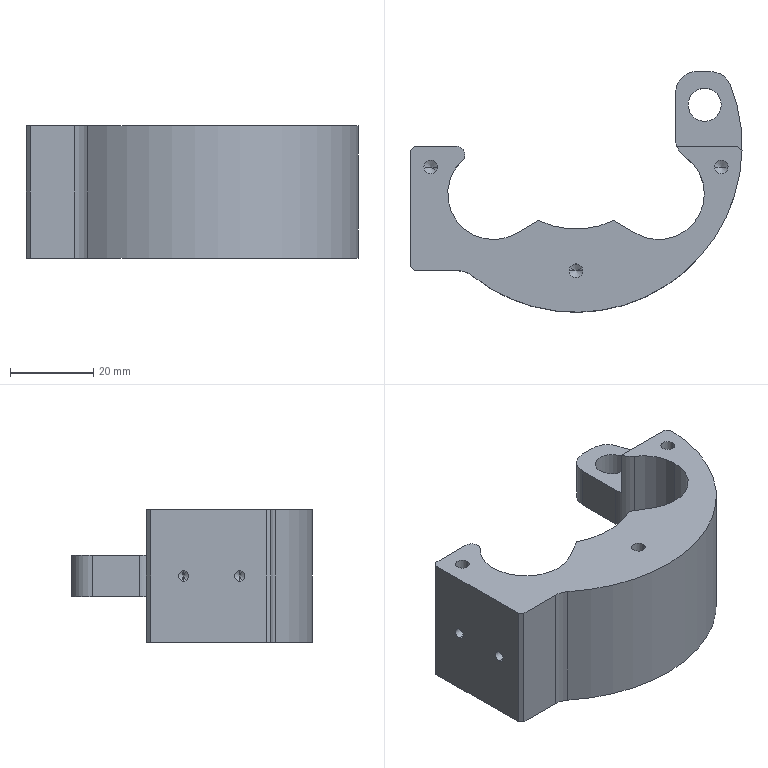Part | STEP file | Support intermediate piece-lower | 1 solid | 62 faces | box 80 x 58 x 32 mm | volume 47494 mm3 | cylinder 29 | plane 17 | cone 16 | commonest cylinder face diameters 3.3 x12 2.5 x4 10 x4 22 x3 4 x2 8 x2